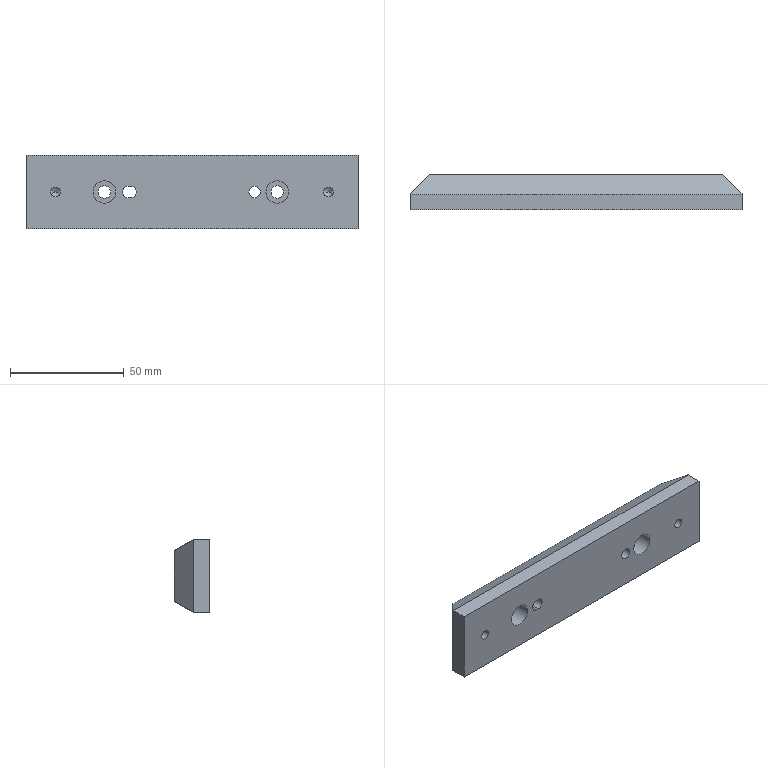NC program | NX | posted with a generic post | part box 146 x 15.5 x 32.5 mm
Whole program:
N10 G17 G21 G94 G90
(FLOOR_WALL , TOOL : D80)
N12 T19 M6
N14 G54
N16 G17 G0 G90 X-45. Y-16.25 S6500 M3
N18 G43 Z30. H19
N20 Z3.
N22 G94 G1 Z0. F1500.
N24 X-42.
N26 X188.
N28 X191.
N30 Z3.
N32 G0 Z30.
N34 M5
(ZLEVEL_PROFILE , TOOL : D10)
N36 T15 M6
N38 G54
N40 G17 G0 G90 X-1.436 Y-37.381 S9500 M3
N42 G43 Z30. H15
N44 Z1.5
N46 G94 G1 X-1.898 Y-37.266 Z1.475 F1000.
N48 X-3.104 Y-36.584 Z1.402
N50 X-4.084 Y-35.604 Z1.33
N52 X-4.766 Y-34.398 Z1.257
N54 X-5.1 Y-33.054 Z1.185
N56 Y0.554 Z-0.577
N58 X-4.766 Y1.898 Z-0.649
N60 X-4.084 Y3.104 Z-0.722
N62 X-3.104 Y4.084 Z-0.795
N64 X-1.898 Y4.766 Z-0.867
N66 X-0.554 Y5.1 Z-0.94
N68 X0. Z-0.969
N70 X146. F3000.
N72 G2 X151.1 Y0. R5.1
N74 G1 Y-32.5
N76 G2 X146. Y-37.6 R5.1
N78 G1 X0.
N80 G2 X-5.1 Y-32.5 R5.1
N82 G1 Y0.
N84 G2 X0. Y5.1 R5.1
N86 G1 X146. Z-1.332
N88 X146.5 Y5.075 Z-1.334
N90 X146.995 Y5.002 Z-1.335
N92 X147.48 Y4.88 Z-1.336
N94 X147.952 Y4.712 Z-1.337
N96 X148.404 Y4.498 Z-1.339
N98 X148.833 Y4.24 Z-1.34
N100 X149.235 Y3.942 Z-1.341
N102 X149.606 Y3.606 Z-1.342
N104 X149.942 Y3.235 Z-1.344
N106 X150.24 Y2.833 Z-1.345
N108 X150.498 Y2.404 Z-1.346
N110 X150.712 Y1.952 Z-1.347
N112 X150.88 Y1.48 Z-1.349
N114 X151.002 Y0.995 Z-1.35
N116 X151.075 Y0.5 Z-1.351
N118 X151.1 Y0. Z-1.352
N120 Y-32.5 Z-1.433
N122 X151.075 Y-33. Z-1.434
N124 X151.002 Y-33.495 Z-1.436
N126 X150.88 Y-33.98 Z-1.437
N128 X150.712 Y-34.452 Z-1.438
N130 X150.498 Y-34.904 Z-1.439
N132 X150.24 Y-35.333 Z-1.441
N134 X149.942 Y-35.735 Z-1.442
N136 X149.606 Y-36.106 Z-1.443
N138 X149.235 Y-36.442 Z-1.444
N140 X148.833 Y-36.74 Z-1.446
N142 X148.404 Y-36.998 Z-1.447
N144 X147.952 Y-37.212 Z-1.448
N146 X147.48 Y-37.38 Z-1.449
N148 X146.995 Y-37.502 Z-1.451
N150 X146.5 Y-37.575 Z-1.452
N152 X146. Y-37.6 Z-1.453
N154 X0. Z-1.817
N156 X-0.5 Y-37.575 Z-1.818
N158 X-0.995 Y-37.502 Z-1.819
N160 X-1.48 Y-37.38 Z-1.82
N162 X-1.952 Y-37.212 Z-1.822
N164 X-2.404 Y-36.998 Z-1.823
N166 X-2.833 Y-36.74 Z-1.824
N168 X-3.235 Y-36.442 Z-1.825
N170 X-3.606 Y-36.106 Z-1.827
N172 X-3.942 Y-35.735 Z-1.828
N174 X-4.24 Y-35.333 Z-1.829
N176 X-4.498 Y-34.904 Z-1.83
N178 X-4.712 Y-34.452 Z-1.832
N180 X-4.88 Y-33.98 Z-1.833
N182 X-5.002 Y-33.495 Z-1.834
N184 X-5.075 Y-33. Z-1.835
N186 X-5.1 Y-32.5 Z-1.837
N188 Y0. Z-1.918
N190 X-5.075 Y0.5 Z-1.919
N192 X-5.002 Y0.995 Z-1.92
N194 X-4.88 Y1.48 Z-1.921
N196 X-4.712 Y1.952 Z-1.923
N198 X-4.498 Y2.404 Z-1.924
N200 X-4.24 Y2.833 Z-1.925
N202 X-3.942 Y3.235 Z-1.926
N204 X-3.606 Y3.606 Z-1.928
N206 X-3.235 Y3.942 Z-1.929
N208 X-2.833 Y4.24 Z-1.93
N210 X-2.404 Y4.498 Z-1.931
N212 X-1.952 Y4.712 Z-1.933
N214 X-1.48 Y4.88 Z-1.934
N216 X-0.995 Y5.002 Z-1.935
N218 X-0.5 Y5.075 Z-1.936
N220 X0. Y5.1 Z-1.938
N222 X146. Z-2.301
N224 X146.5 Y5.075 Z-2.302
N226 X146.995 Y5.002 Z-2.304
N228 X147.48 Y4.88 Z-2.305
N230 X147.952 Y4.712 Z-2.306
N232 X148.404 Y4.498 Z-2.307
N234 X148.833 Y4.24 Z-2.309
N236 X149.235 Y3.942 Z-2.31
N238 X149.606 Y3.606 Z-2.311
N240 X149.942 Y3.235 Z-2.312
N242 X150.24 Y2.833 Z-2.314
N244 X150.498 Y2.404 Z-2.315
N246 X150.712 Y1.952 Z-2.316
N248 X150.88 Y1.48 Z-2.317
N250 X151.002 Y0.995 Z-2.319
N252 X151.075 Y0.5 Z-2.32
N254 X151.1 Y0. Z-2.321
N256 Y-32.5 Z-2.402
N258 X151.075 Y-33. Z-2.403
N260 X151.002 Y-33.495 Z-2.404
N262 X150.88 Y-33.98 Z-2.406
N264 X150.712 Y-34.452 Z-2.407
N266 X150.498 Y-34.904 Z-2.408
N268 X150.24 Y-35.333 Z-2.409
N270 X149.942 Y-35.735 Z-2.411
N272 X149.606 Y-36.106 Z-2.412
N274 X149.235 Y-36.442 Z-2.413
N276 X148.833 Y-36.74 Z-2.414
N278 X148.404 Y-36.998 Z-2.416
N280 X147.952 Y-37.212 Z-2.417
N282 X147.48 Y-37.38 Z-2.418
N284 X146.995 Y-37.502 Z-2.419
N286 X146.5 Y-37.575 Z-2.421
N288 X146. Y-37.6 Z-2.422
N290 X0. Z-2.785
N292 X-0.5 Y-37.575 Z-2.787
N294 X-0.995 Y-37.502 Z-2.788
N296 X-1.48 Y-37.38 Z-2.789
N298 X-1.952 Y-37.212 Z-2.79
N300 X-2.404 Y-36.998 Z-2.792
N302 X-2.833 Y-36.74 Z-2.793
N304 X-3.235 Y-36.442 Z-2.794
N306 X-3.606 Y-36.106 Z-2.795
N308 X-3.942 Y-35.735 Z-2.797
N310 X-4.24 Y-35.333 Z-2.798
N312 X-4.498 Y-34.904 Z-2.799
N314 X-4.712 Y-34.452 Z-2.8
N316 X-4.88 Y-33.98 Z-2.802
N318 X-5.002 Y-33.495 Z-2.803
N320 X-5.075 Y-33. Z-2.804
N322 X-5.1 Y-32.5 Z-2.805
N324 Y0. Z-2.886
N326 X-5.075 Y0.5 Z-2.888
N328 X-5.002 Y0.995 Z-2.889
N330 X-4.88 Y1.48 Z-2.89
N332 X-4.712 Y1.952 Z-2.891
N334 X-4.498 Y2.404 Z-2.893
N336 X-4.24 Y2.833 Z-2.894
N338 X-3.942 Y3.235 Z-2.895
N340 X-3.606 Y3.606 Z-2.896
N342 X-3.235 Y3.942 Z-2.898
N344 X-2.833 Y4.24 Z-2.899
N346 X-2.404 Y4.498 Z-2.9
N348 X-1.952 Y4.712 Z-2.901
N350 X-1.48 Y4.88 Z-2.903
N352 X-0.995 Y5.002 Z-2.904
N354 X-0.5 Y5.075 Z-2.905
N356 X0. Y5.1 Z-2.906
N358 X146. Z-3.27
N360 X146.5 Y5.075 Z-3.271
N362 X146.995 Y5.002 Z-3.272
N364 X147.48 Y4.88 Z-3.274
N366 X147.952 Y4.712 Z-3.275
N368 X148.404 Y4.498 Z-3.276
N370 X148.833 Y4.24 Z-3.277
N372 X149.235 Y3.942 Z-3.279
N374 X149.606 Y3.606 Z-3.28
N376 X149.942 Y3.235 Z-3.281
N378 X150.24 Y2.833 Z-3.282
N380 X150.498 Y2.404 Z-3.284
N382 X150.712 Y1.952 Z-3.285
N384 X150.88 Y1.48 Z-3.286
N386 X151.002 Y0.995 Z-3.287
N388 X151.075 Y0.5 Z-3.289
N390 X151.1 Y0. Z-3.29
N392 Y-32.5 Z-3.371
N394 X151.075 Y-33. Z-3.372
N396 X151.002 Y-33.495 Z-3.373
N398 X150.88 Y-33.98 Z-3.374
N400 X150.712 Y-34.452 Z-3.376
N402 X150.498 Y-34.904 Z-3.377
N404 X150.24 Y-35.333 Z-3.378
N406 X149.942 Y-35.735 Z-3.379
N408 X149.606 Y-36.106 Z-3.381
N410 X149.235 Y-36.442 Z-3.382
N412 X148.833 Y-36.74 Z-3.383
N414 X148.404 Y-36.998 Z-3.384
N416 X147.952 Y-37.212 Z-3.386
N418 X147.48 Y-37.38 Z-3.387
N420 X146.995 Y-37.502 Z-3.388
N422 X146.5 Y-37.575 Z-3.389
N424 X146. Y-37.6 Z-3.391
N426 X0. Z-3.754
N428 X-0.5 Y-37.575 Z-3.755
N430 X-0.995 Y-37.502 Z-3.757
N432 X-1.48 Y-37.38 Z-3.758
N434 X-1.952 Y-37.212 Z-3.759
N436 X-2.404 Y-36.998 Z-3.76
N438 X-2.833 Y-36.74 Z-3.762
N440 X-3.235 Y-36.442 Z-3.763
N442 X-3.606 Y-36.106 Z-3.764
N444 X-3.942 Y-35.735 Z-3.765
N446 X-4.24 Y-35.333 Z-3.767
N448 X-4.498 Y-34.904 Z-3.768
N450 X-4.712 Y-34.452 Z-3.769
N452 X-4.88 Y-33.98 Z-3.77
N454 X-5.002 Y-33.495 Z-3.772
N456 X-5.075 Y-33. Z-3.773
N458 X-5.1 Y-32.5 Z-3.774
N460 Y0. Z-3.855
N462 X-5.075 Y0.5 Z-3.856
N464 X-5.002 Y0.995 Z-3.858
N466 X-4.88 Y1.48 Z-3.859
N468 X-4.712 Y1.952 Z-3.86
N470 X-4.498 Y2.404 Z-3.861
N472 X-4.24 Y2.833 Z-3.863
N474 X-3.942 Y3.235 Z-3.864
N476 X-3.606 Y3.606 Z-3.865
N478 X-3.235 Y3.942 Z-3.866
N480 X-2.833 Y4.24 Z-3.868
N482 X-2.404 Y4.498 Z-3.869
N484 X-1.952 Y4.712 Z-3.87
N486 X-1.48 Y4.88 Z-3.871
N488 X-0.995 Y5.002 Z-3.873
N490 X-0.5 Y5.075 Z-3.874
N492 X0. Y5.1 Z-3.875
N494 X146. Z-4.239
N496 X146.5 Y5.075 Z-4.24
N498 X146.995 Y5.002 Z-4.241
N500 X147.48 Y4.88 Z-4.242
N502 X147.952 Y4.712 Z-4.244
N504 X148.404 Y4.498 Z-4.245
N506 X148.833 Y4.24 Z-4.246
N508 X149.235 Y3.942 Z-4.247
N510 X149.606 Y3.606 Z-4.249
N512 X149.942 Y3.235 Z-4.25
N514 X150.24 Y2.833 Z-4.251
N516 X150.498 Y2.404 Z-4.252
N518 X150.712 Y1.952 Z-4.254
N520 X150.88 Y1.48 Z-4.255
N522 X151.002 Y0.995 Z-4.256
N524 X151.075 Y0.5 Z-4.257
N526 X151.1 Y0. Z-4.259
N528 Y-32.5 Z-4.339
N530 X151.075 Y-33. Z-4.341
N532 X151.002 Y-33.495 Z-4.342
N534 X150.88 Y-33.98 Z-4.343
N536 X150.712 Y-34.452 Z-4.344
N538 X150.498 Y-34.904 Z-4.346
N540 X150.24 Y-35.333 Z-4.347
N542 X149.942 Y-35.735 Z-4.348
N544 X149.606 Y-36.106 Z-4.349
N546 X149.235 Y-36.442 Z-4.351
N548 X148.833 Y-36.74 Z-4.352
N550 X148.404 Y-36.998 Z-4.353
N552 X147.952 Y-37.212 Z-4.354
N554 X147.48 Y-37.38 Z-4.356
N556 X146.995 Y-37.502 Z-4.357
N558 X146.5 Y-37.575 Z-4.358
N560 X146. Y-37.6 Z-4.359
N562 X0. Z-4.723
N564 X-0.5 Y-37.575 Z-4.724
N566 X-0.995 Y-37.502 Z-4.725
N568 X-1.48 Y-37.38 Z-4.727
N570 X-1.952 Y-37.212 Z-4.728
N572 X-2.404 Y-36.998 Z-4.729
N574 X-2.833 Y-36.74 Z-4.73
N576 X-3.235 Y-36.442 Z-4.732
N578 X-3.606 Y-36.106 Z-4.733
N580 X-3.942 Y-35.735 Z-4.734
N582 X-4.24 Y-35.333 Z-4.735
N584 X-4.498 Y-34.904 Z-4.737
N586 X-4.712 Y-34.452 Z-4.738
N588 X-4.88 Y-33.98 Z-4.739
N590 X-5.002 Y-33.495 Z-4.74
N592 X-5.075 Y-33. Z-4.742
N594 X-5.1 Y-32.5 Z-4.743
N596 Y0. Z-4.824
N598 X-5.075 Y0.5 Z-4.825
N600 X-5.002 Y0.995 Z-4.826
N602 X-4.88 Y1.48 Z-4.828
N604 X-4.712 Y1.952 Z-4.829
N606 X-4.498 Y2.404 Z-4.83
N608 X-4.24 Y2.833 Z-4.831
N610 X-3.942 Y3.235 Z-4.833
N612 X-3.606 Y3.606 Z-4.834
N614 X-3.235 Y3.942 Z-4.835
N616 X-2.833 Y4.24 Z-4.836
N618 X-2.404 Y4.498 Z-4.838
N620 X-1.952 Y4.712 Z-4.839
N622 X-1.48 Y4.88 Z-4.84
N624 X-0.995 Y5.002 Z-4.841
N626 X-0.5 Y5.075 Z-4.843
N628 X0. Y5.1 Z-4.844
N630 X146. Z-5.207
N632 X146.5 Y5.075 Z-5.209
N634 X146.995 Y5.002 Z-5.21
N636 X147.48 Y4.88 Z-5.211
N638 X147.952 Y4.712 Z-5.212
N640 X148.404 Y4.498 Z-5.214
N642 X148.833 Y4.24 Z-5.215
N644 X149.235 Y3.942 Z-5.216
N646 X149.606 Y3.606 Z-5.217
N648 X149.942 Y3.235 Z-5.219
N650 X150.24 Y2.833 Z-5.22
N652 X150.498 Y2.404 Z-5.221
N654 X150.712 Y1.952 Z-5.222
N656 X150.88 Y1.48 Z-5.224
N658 X151.002 Y0.995 Z-5.225
N660 X151.075 Y0.5 Z-5.226
N662 X151.1 Y0. Z-5.227
N664 Y-32.5 Z-5.308
N666 X151.075 Y-33. Z-5.309
N668 X151.002 Y-33.495 Z-5.311
N670 X150.88 Y-33.98 Z-5.312
N672 X150.712 Y-34.452 Z-5.313
N674 X150.498 Y-34.904 Z-5.314
N676 X150.24 Y-35.333 Z-5.316
N678 X149.942 Y-35.735 Z-5.317
N680 X149.606 Y-36.106 Z-5.318
N682 X149.235 Y-36.442 Z-5.319
N684 X148.833 Y-36.74 Z-5.321
N686 X148.404 Y-36.998 Z-5.322
N688 X147.952 Y-37.212 Z-5.323
N690 X147.48 Y-37.38 Z-5.324
N692 X146.995 Y-37.502 Z-5.326
N694 X146.5 Y-37.575 Z-5.327
N696 X146. Y-37.6 Z-5.328
N698 X0. Z-5.692
N700 X-0.5 Y-37.575 Z-5.693
N702 X-0.995 Y-37.502 Z-5.694
N704 X-1.48 Y-37.38 Z-5.695
N706 X-1.952 Y-37.212 Z-5.697
N708 X-2.404 Y-36.998 Z-5.698
N710 X-2.833 Y-36.74 Z-5.699
N712 X-3.235 Y-36.442 Z-5.7
N714 X-3.606 Y-36.106 Z-5.702
N716 X-3.942 Y-35.735 Z-5.703
N718 X-4.24 Y-35.333 Z-5.704
N720 X-4.498 Y-34.904 Z-5.705
N722 X-4.712 Y-34.452 Z-5.707
N724 X-4.88 Y-33.98 Z-5.708
N726 X-5.002 Y-33.495 Z-5.709
N728 X-5.075 Y-33. Z-5.71
N730 X-5.1 Y-32.5 Z-5.712
N732 Y0. Z-5.793
N734 X-5.075 Y0.5 Z-5.794
N736 X-5.002 Y0.995 Z-5.795
N738 X-4.88 Y1.48 Z-5.796
N740 X-4.712 Y1.952 Z-5.798
N742 X-4.498 Y2.404 Z-5.799
N744 X-4.24 Y2.833 Z-5.8
N746 X-3.942 Y3.235 Z-5.801
N748 X-3.606 Y3.606 Z-5.803
N750 X-3.235 Y3.942 Z-5.804
N752 X-2.833 Y4.24 Z-5.805
N754 X-2.404 Y4.498 Z-5.806
N756 X-1.952 Y4.712 Z-5.808
N758 X-1.48 Y4.88 Z-5.809
N760 X-0.995 Y5.002 Z-5.81
N762 X-0.5 Y5.075 Z-5.811
N764 X0. Y5.1 Z-5.813
N766 X146. Z-6.176
N768 X146.5 Y5.075 Z-6.177
N770 X146.995 Y5.002 Z-6.179
N772 X147.48 Y4.88 Z-6.18
N774 X147.952 Y4.712 Z-6.181
N776 X148.404 Y4.498 Z-6.182
N778 X148.833 Y4.24 Z-6.184
N780 X149.235 Y3.942 Z-6.185
N782 X149.606 Y3.606 Z-6.186
N784 X149.942 Y3.235 Z-6.187
N786 X150.24 Y2.833 Z-6.189
N788 X150.498 Y2.404 Z-6.19
N790 X150.712 Y1.952 Z-6.191
N792 X150.88 Y1.48 Z-6.192
N794 X151.002 Y0.995 Z-6.194
N796 X151.075 Y0.5 Z-6.195
N798 X151.1 Y0. Z-6.196
N800 Y-32.5 Z-6.277
N802 X151.075 Y-33. Z-6.278
N804 X151.002 Y-33.495 Z-6.279
N806 X150.88 Y-33.98 Z-6.281
N808 X150.712 Y-34.452 Z-6.282
N810 X150.498 Y-34.904 Z-6.283
N812 X150.24 Y-35.333 Z-6.284
N814 X149.942 Y-35.735 Z-6.286
N816 X149.606 Y-36.106 Z-6.287
N818 X149.235 Y-36.442 Z-6.288
N820 X148.833 Y-36.74 Z-6.289
N822 X148.404 Y-36.998 Z-6.291
N824 X147.952 Y-37.212 Z-6.292
N826 X147.48 Y-37.38 Z-6.293
N828 X146.995 Y-37.502 Z-6.294
N830 X146.5 Y-37.575 Z-6.296
N832 X146. Y-37.6 Z-6.297
N834 X0. Z-6.66
N836 X-0.5 Y-37.575 Z-6.662
N838 X-0.995 Y-37.502 Z-6.663
N840 X-1.48 Y-37.38 Z-6.664
N842 X-1.952 Y-37.212 Z-6.665
N844 X-2.404 Y-36.998 Z-6.667
N846 X-2.833 Y-36.74 Z-6.668
N848 X-3.235 Y-36.442 Z-6.669
N850 X-3.606 Y-36.106 Z-6.67
N852 X-3.942 Y-35.735 Z-6.672
N854 X-4.24 Y-35.333 Z-6.673
N856 X-4.498 Y-34.904 Z-6.674
N858 X-4.712 Y-34.452 Z-6.675
N860 X-4.88 Y-33.98 Z-6.677
N862 X-5.002 Y-33.495 Z-6.678
N864 X-5.075 Y-33. Z-6.679
N866 X-5.1 Y-32.5 Z-6.68
N868 Y0. Z-6.761
N870 X-5.075 Y0.5 Z-6.763
N872 X-5.002 Y0.995 Z-6.764
N874 X-4.88 Y1.48 Z-6.765
N876 X-4.712 Y1.952 Z-6.766
N878 X-4.498 Y2.404 Z-6.768
N880 X-4.24 Y2.833 Z-6.769
N882 X-3.942 Y3.235 Z-6.77
N884 X-3.606 Y3.606 Z-6.771
N886 X-3.235 Y3.942 Z-6.773
N888 X-2.833 Y4.24 Z-6.774
N890 X-2.404 Y4.498 Z-6.775
N892 X-1.952 Y4.712 Z-6.776
N894 X-1.48 Y4.88 Z-6.778
N896 X-0.995 Y5.002 Z-6.779
N898 X-0.5 Y5.075 Z-6.78
N900 X0. Y5.1 Z-6.781
N902 X146. Z-7.145
N904 X146.5 Y5.075 Z-7.146
N906 X146.995 Y5.002 Z-7.147
N908 X147.48 Y4.88 Z-7.149
N910 X147.952 Y4.712 Z-7.15
N912 X148.404 Y4.498 Z-7.151
N914 X148.833 Y4.24 Z-7.152
N916 X149.235 Y3.942 Z-7.154
N918 X149.606 Y3.606 Z-7.155
N920 X149.942 Y3.235 Z-7.156
N922 X150.24 Y2.833 Z-7.157
N924 X150.498 Y2.404 Z-7.159
N926 X150.712 Y1.952 Z-7.16
N928 X150.88 Y1.48 Z-7.161
N930 X151.002 Y0.995 Z-7.162
N932 X151.075 Y0.5 Z-7.164
N934 X151.1 Y0. Z-7.165
N936 Y-32.5 Z-7.246
N938 X151.075 Y-33. Z-7.247
N940 X151.002 Y-33.495 Z-7.248
N942 X150.88 Y-33.98 Z-7.249
N944 X150.712 Y-34.452 Z-7.251
N946 X150.498 Y-34.904 Z-7.252
N948 X150.24 Y-35.333 Z-7.253
N950 X149.942 Y-35.735 Z-7.254
N952 X149.606 Y-36.106 Z-7.256
N954 X149.235 Y-36.442 Z-7.257
N956 X148.833 Y-36.74 Z-7.258
N958 X148.404 Y-36.998 Z-7.259
N960 X147.952 Y-37.212 Z-7.261
N962 X147.48 Y-37.38 Z-7.262
N964 X146.995 Y-37.502 Z-7.263
N966 X146.5 Y-37.575 Z-7.264
N968 X146. Y-37.6 Z-7.266
N970 X0. Z-7.629
N972 X-0.5 Y-37.575 Z-7.63
N974 X-0.995 Y-37.502 Z-7.632
N976 X-1.48 Y-37.38 Z-7.633
N978 X-1.952 Y-37.212 Z-7.634
N980 X-2.404 Y-36.998 Z-7.635
N982 X-2.833 Y-36.74 Z-7.637
N984 X-3.235 Y-36.442 Z-7.638
N986 X-3.606 Y-36.106 Z-7.639
N988 X-3.942 Y-35.735 Z-7.64
N990 X-4.24 Y-35.333 Z-7.642
N992 X-4.498 Y-34.904 Z-7.643
N994 X-4.712 Y-34.452 Z-7.644
N996 X-4.88 Y-33.98 Z-7.645
N998 X-5.002 Y-33.495 Z-7.647
N1000 X-5.075 Y-33. Z-7.648
N1002 X-5.1 Y-32.5 Z-7.649
N1004 Y0. Z-7.73
N1006 X-5.075 Y0.5 Z-7.731
N1008 X-5.002 Y0.995 Z-7.733
N1010 X-4.88 Y1.48 Z-7.734
N1012 X-4.712 Y1.952 Z-7.735
N1014 X-4.498 Y2.404 Z-7.736
N1016 X-4.24 Y2.833 Z-7.738
N1018 X-3.942 Y3.235 Z-7.739
N1020 X-3.606 Y3.606 Z-7.74
N1022 X-3.235 Y3.942 Z-7.741
N1024 X-2.833 Y4.24 Z-7.743
N1026 X-2.404 Y4.498 Z-7.744
N1028 X-1.952 Y4.712 Z-7.745
N1030 X-1.48 Y4.88 Z-7.746
N1032 X-0.995 Y5.002 Z-7.748
N1034 X-0.5 Y5.075 Z-7.749
N1036 X0. Y5.1 Z-7.75
N1038 X146. Z-8.114
N1040 X146.5 Y5.075 Z-8.115
N1042 X146.995 Y5.002 Z-8.116
N1044 X147.48 Y4.88 Z-8.117
N1046 X147.952 Y4.712 Z-8.119
N1048 X148.404 Y4.498 Z-8.12
N1050 X148.833 Y4.24 Z-8.121
N1052 X149.235 Y3.942 Z-8.122
N1054 X149.606 Y3.606 Z-8.124
N1056 X149.942 Y3.235 Z-8.125
N1058 X150.24 Y2.833 Z-8.126
N1060 X150.498 Y2.404 Z-8.127
N1062 X150.712 Y1.952 Z-8.129
N1064 X150.88 Y1.48 Z-8.13
N1066 X151.002 Y0.995 Z-8.131
N1068 X151.075 Y0.5 Z-8.132
N1070 X151.1 Y0. Z-8.134
N1072 Y-32.5 Z-8.214
N1074 X151.075 Y-33. Z-8.216
N1076 X151.002 Y-33.495 Z-8.217
N1078 X150.88 Y-33.98 Z-8.218
N1080 X150.712 Y-34.452 Z-8.219
N1082 X150.498 Y-34.904 Z-8.221
N1084 X150.24 Y-35.333 Z-8.222
N1086 X149.942 Y-35.735 Z-8.223
N1088 X149.606 Y-36.106 Z-8.224
N1090 X149.235 Y-36.442 Z-8.226
N1092 X148.833 Y-36.74 Z-8.227
N1094 X148.404 Y-36.998 Z-8.228
N1096 X147.952 Y-37.212 Z-8.229
N1098 X147.48 Y-37.38 Z-8.231
N1100 X146.995 Y-37.502 Z-8.232
N1102 X146.5 Y-37.575 Z-8.233
N1104 X146. Y-37.6 Z-8.234
N1106 X0. Z-8.598
N1108 X-0.5 Y-37.575 Z-8.599
N1110 X-0.995 Y-37.502 Z-8.6
N1112 X-1.48 Y-37.38 Z-8.602
N1114 X-1.952 Y-37.212 Z-8.603
N1116 X-2.404 Y-36.998 Z-8.604
N1118 X-2.833 Y-36.74 Z-8.605
N1120 X-3.235 Y-36.442 Z-8.607
N1122 X-3.606 Y-36.106 Z-8.608
N1124 X-3.942 Y-35.735 Z-8.609
N1126 X-4.24 Y-35.333 Z-8.61
N1128 X-4.498 Y-34.904 Z-8.612
N1130 X-4.712 Y-34.452 Z-8.613
N1132 X-4.88 Y-33.98 Z-8.614
N1134 X-5.002 Y-33.495 Z-8.615
N1136 X-5.075 Y-33. Z-8.617
N1138 X-5.1 Y-32.5 Z-8.618
N1140 Y0. Z-8.699
N1142 X-5.075 Y0.5 Z-8.7
N1144 X-5.002 Y0.995 Z-8.701
N1146 X-4.88 Y1.48 Z-8.703
N1148 X-4.712 Y1.952 Z-8.704
N1150 X-4.498 Y2.404 Z-8.705
N1152 X-4.24 Y2.833 Z-8.706
N1154 X-3.942 Y3.235 Z-8.708
N1156 X-3.606 Y3.606 Z-8.709
N1158 X-3.235 Y3.942 Z-8.71
N1160 X-2.833 Y4.24 Z-8.711
N1162 X-2.404 Y4.498 Z-8.713
N1164 X-1.952 Y4.712 Z-8.714
N1166 X-1.48 Y4.88 Z-8.715
N1168 X-0.995 Y5.002 Z-8.716
N1170 X-0.5 Y5.075 Z-8.718
N1172 X0. Y5.1 Z-8.719
N1174 X146. Z-9.082
N1176 X146.5 Y5.075 Z-9.084
N1178 X146.995 Y5.002 Z-9.085
N1180 X147.48 Y4.88 Z-9.086
N1182 X147.952 Y4.712 Z-9.087
N1184 X148.404 Y4.498 Z-9.089
N1186 X148.833 Y4.24 Z-9.09
N1188 X149.235 Y3.942 Z-9.091
N1190 X149.606 Y3.606 Z-9.092
N1192 X149.942 Y3.235 Z-9.094
N1194 X150.24 Y2.833 Z-9.095
N1196 X150.498 Y2.404 Z-9.096
N1198 X150.712 Y1.952 Z-9.097
N1200 X150.88 Y1.48 Z-9.099
N1202 X151.002 Y0.995 Z-9.1
N1204 X151.075 Y0.5 Z-9.101
N1206 X151.1 Y0. Z-9.102
N1208 Y-32.5 Z-9.183
N1210 X151.075 Y-33. Z-9.184
N1212 X151.002 Y-33.495 Z-9.186
N1214 X150.88 Y-33.98 Z-9.187
N1216 X150.712 Y-34.452 Z-9.188
N1218 X150.498 Y-34.904 Z-9.189
N1220 X150.24 Y-35.333 Z-9.191
N1222 X149.942 Y-35.735 Z-9.192
N1224 X149.606 Y-36.106 Z-9.193
N1226 X149.235 Y-36.442 Z-9.194
N1228 X148.833 Y-36.74 Z-9.196
N1230 X148.404 Y-36.998 Z-9.197
N1232 X147.952 Y-37.212 Z-9.198
N1234 X147.48 Y-37.38 Z-9.199
N1236 X146.995 Y-37.502 Z-9.201
N1238 X146.5 Y-37.575 Z-9.202
N1240 X146. Y-37.6 Z-9.203
N1242 X0. Z-9.567
N1244 X-0.5 Y-37.575 Z-9.568
N1246 X-0.995 Y-37.502 Z-9.569
N1248 X-1.48 Y-37.38 Z-9.57
N1250 X-1.952 Y-37.212 Z-9.572
N1252 X-2.404 Y-36.998 Z-9.573
N1254 X-2.833 Y-36.74 Z-9.574
N1256 X-3.235 Y-36.442 Z-9.575
N1258 X-3.606 Y-36.106 Z-9.577
N1260 X-3.942 Y-35.735 Z-9.578
N1262 X-4.24 Y-35.333 Z-9.579
N1264 X-4.498 Y-34.904 Z-9.58
N1266 X-4.712 Y-34.452 Z-9.582
N1268 X-4.88 Y-33.98 Z-9.583
N1270 X-5.002 Y-33.495 Z-9.584
N1272 X-5.075 Y-33. Z-9.585
N1274 X-5.1 Y-32.5 Z-9.587
N1276 Y0. Z-9.668
N1278 X-5.075 Y0.5 Z-9.669
N1280 X-5.002 Y0.995 Z-9.67
N1282 X-4.88 Y1.48 Z-9.671
N1284 X-4.712 Y1.952 Z-9.673
N1286 X-4.498 Y2.404 Z-9.674
N1288 X-4.24 Y2.833 Z-9.675
N1290 X-3.942 Y3.235 Z-9.676
N1292 X-3.606 Y3.606 Z-9.678
N1294 X-3.235 Y3.942 Z-9.679
N1296 X-2.833 Y4.24 Z-9.68
N1298 X-2.404 Y4.498 Z-9.681
N1300 X-1.952 Y4.712 Z-9.683
N1302 X-1.48 Y4.88 Z-9.684
N1304 X-0.995 Y5.002 Z-9.685
N1306 X-0.5 Y5.075 Z-9.686
N1308 X0. Y5.1 Z-9.688
N1310 X146. Z-10.051
N1312 X146.5 Y5.075 Z-10.052
N1314 X146.995 Y5.002 Z-10.054
N1316 X147.48 Y4.88 Z-10.055
N1318 X147.952 Y4.712 Z-10.056
N1320 X148.404 Y4.498 Z-10.057
N1322 X148.833 Y4.24 Z-10.059
N1324 X149.235 Y3.942 Z-10.06
N1326 X149.606 Y3.606 Z-10.061
N1328 X149.942 Y3.235 Z-10.062
N1330 X150.24 Y2.833 Z-10.064
N1332 X150.498 Y2.404 Z-10.065
N1334 X150.712 Y1.952 Z-10.066
N1336 X150.88 Y1.48 Z-10.067
N1338 X151.002 Y0.995 Z-10.069
N1340 X151.075 Y0.5 Z-10.07
N1342 X151.1 Y0. Z-10.071
N1344 Y-32.5 Z-10.152
N1346 X151.075 Y-33. Z-10.153
N1348 X151.002 Y-33.495 Z-10.154
N1350 X150.88 Y-33.98 Z-10.156
N1352 X150.712 Y-34.452 Z-10.157
N1354 X150.498 Y-34.904 Z-10.158
N1356 X150.24 Y-35.333 Z-10.159
N1358 X149.942 Y-35.735 Z-10.161
N1360 X149.606 Y-36.106 Z-10.162
N1362 X149.235 Y-36.442 Z-10.163
N1364 X148.833 Y-36.74 Z-10.164
N1366 X148.404 Y-36.998 Z-10.166
N1368 X147.952 Y-37.212 Z-10.167
N1370 X147.48 Y-37.38 Z-10.168
N1372 X146.995 Y-37.502 Z-10.169
N1374 X146.5 Y-37.575 Z-10.171
N1376 X146. Y-37.6 Z-10.172
N1378 X0. Z-10.535
N1380 X-0.5 Y-37.575 Z-10.537
N1382 X-0.995 Y-37.502 Z-10.538
N1384 X-1.48 Y-37.38 Z-10.539
N1386 X-1.952 Y-37.212 Z-10.54
N1388 X-2.404 Y-36.998 Z-10.542
N1390 X-2.833 Y-36.74 Z-10.543
N1392 X-3.235 Y-36.442 Z-10.544
N1394 X-3.606 Y-36.106 Z-10.545
N1396 X-3.942 Y-35.735 Z-10.547
N1398 X-4.24 Y-35.333 Z-10.548
N1400 X-4.498 Y-34.904 Z-10.549
N1402 X-4.712 Y-34.452 Z-10.55
N1404 X-4.88 Y-33.98 Z-10.552
N1406 X-5.002 Y-33.495 Z-10.553
N1408 X-5.075 Y-33. Z-10.554
N1410 X-5.1 Y-32.5 Z-10.555
N1412 Y0. Z-10.636
N1414 X-5.075 Y0.5 Z-10.638
N1416 X-5.002 Y0.995 Z-10.639
N1418 X-4.88 Y1.48 Z-10.64
N1420 X-4.712 Y1.952 Z-10.641
N1422 X-4.498 Y2.404 Z-10.643
N1424 X-4.24 Y2.833 Z-10.644
N1426 X-3.942 Y3.235 Z-10.645
N1428 X-3.606 Y3.606 Z-10.646
N1430 X-3.235 Y3.942 Z-10.648
N1432 X-2.833 Y4.24 Z-10.649
N1434 X-2.404 Y4.498 Z-10.65
N1436 X-1.952 Y4.712 Z-10.651
N1438 X-1.48 Y4.88 Z-10.653
N1440 X-0.995 Y5.002 Z-10.654
N1442 X-0.5 Y5.075 Z-10.655
N1444 X0. Y5.1 Z-10.656
N1446 X146. Z-11.02
N1448 X146.5 Y5.075 Z-11.021
N1450 X146.995 Y5.002 Z-11.022
N1452 X147.48 Y4.88 Z-11.024
N1454 X147.952 Y4.712 Z-11.025
N1456 X148.404 Y4.498 Z-11.026
N1458 X148.833 Y4.24 Z-11.027
N1460 X149.235 Y3.942 Z-11.029
N1462 X149.606 Y3.606 Z-11.03
N1464 X149.942 Y3.235 Z-11.031
N1466 X150.24 Y2.833 Z-11.032
N1468 X150.498 Y2.404 Z-11.034
N1470 X150.712 Y1.952 Z-11.035
N1472 X150.88 Y1.48 Z-11.036
N1474 X151.002 Y0.995 Z-11.037
N1476 X151.075 Y0.5 Z-11.039
N1478 X151.1 Y0. Z-11.04
N1480 Y-32.5 Z-11.121
N1482 X151.075 Y-33. Z-11.122
N1484 X151.002 Y-33.495 Z-11.123
N1486 X150.88 Y-33.98 Z-11.124
N1488 X150.712 Y-34.452 Z-11.126
N1490 X150.498 Y-34.904 Z-11.127
N1492 X150.24 Y-35.333 Z-11.128
N1494 X149.942 Y-35.735 Z-11.129
N1496 X149.606 Y-36.106 Z-11.131
N1498 X149.235 Y-36.442 Z-11.132
N1500 X148.833 Y-36.74 Z-11.133
N1502 X148.404 Y-36.998 Z-11.134
N1504 X147.952 Y-37.212 Z-11.136
N1506 X147.48 Y-37.38 Z-11.137
N1508 X146.995 Y-37.502 Z-11.138
N1510 X146.5 Y-37.575 Z-11.139
N1512 X146. Y-37.6 Z-11.141
N1514 X0. Z-11.504
N1516 X-0.5 Y-37.575 Z-11.505
N1518 X-0.995 Y-37.502 Z-11.507
N1520 X-1.48 Y-37.38 Z-11.508
N1522 X-1.952 Y-37.212 Z-11.509
N1524 X-2.404 Y-36.998 Z-11.51
N1526 X-2.833 Y-36.74 Z-11.512
N1528 X-3.235 Y-36.442 Z-11.513
N1530 X-3.606 Y-36.106 Z-11.514
N1532 X-3.942 Y-35.735 Z-11.515
N1534 X-4.24 Y-35.333 Z-11.517
N1536 X-4.498 Y-34.904 Z-11.518
N1538 X-4.712 Y-34.452 Z-11.519
N1540 X-4.88 Y-33.98 Z-11.52
N1542 X-5.002 Y-33.495 Z-11.522
N1544 X-5.075 Y-33. Z-11.523
N1546 X-5.1 Y-32.5 Z-11.524
N1548 Y0. Z-11.605
N1550 X-5.075 Y0.5 Z-11.606
N1552 X-5.002 Y0.995 Z-11.608
N1554 X-4.88 Y1.48 Z-11.609
N1556 X-4.712 Y1.952 Z-11.61
N1558 X-4.498 Y2.404 Z-11.611
N1560 X-4.24 Y2.833 Z-11.613
N1562 X-3.942 Y3.235 Z-11.614
N1564 X-3.606 Y3.606 Z-11.615
N1566 X-3.235 Y3.942 Z-11.616
N1568 X-2.833 Y4.24 Z-11.618
N1570 X-2.404 Y4.498 Z-11.619
N1572 X-1.952 Y4.712 Z-11.62
N1574 X-1.48 Y4.88 Z-11.621
N1576 X-0.995 Y5.002 Z-11.623
N1578 X-0.5 Y5.075 Z-11.624
N1580 X0. Y5.1 Z-11.625
N1582 X146. Z-11.989
N1584 X146.5 Y5.075 Z-11.99
N1586 X146.995 Y5.002 Z-11.991
N1588 X147.48 Y4.88 Z-11.992
N1590 X147.952 Y4.712 Z-11.994
N1592 X148.404 Y4.498 Z-11.995
N1594 X148.833 Y4.24 Z-11.996
N1596 X149.235 Y3.942 Z-11.997
N1598 X149.606 Y3.606 Z-11.999
N1600 X149.942 Y3.235 Z-12.
N1602 X150.24 Y2.833 Z-12.001
N1604 X150.498 Y2.404 Z-12.002
N1606 X150.712 Y1.952 Z-12.004
N1608 X150.88 Y1.48 Z-12.005
N1610 X151.002 Y0.995 Z-12.006
N1612 X151.075 Y0.5 Z-12.007
N1614 X151.1 Y0. Z-12.009
N1616 Y-32.5 Z-12.089
N1618 X151.075 Y-33. Z-12.091
N1620 X151.002 Y-33.495 Z-12.092
N1622 X150.88 Y-33.98 Z-12.093
N1624 X150.712 Y-34.452 Z-12.094
N1626 X150.498 Y-34.904 Z-12.096
N1628 X150.24 Y-35.333 Z-12.097
N1630 X149.942 Y-35.735 Z-12.098
N1632 X149.606 Y-36.106 Z-12.099
N1634 X149.235 Y-36.442 Z-12.101
N1636 X148.833 Y-36.74 Z-12.102
N1638 X148.404 Y-36.998 Z-12.103
N1640 X147.952 Y-37.212 Z-12.104
N1642 X147.48 Y-37.38 Z-12.106
N1644 X146.995 Y-37.502 Z-12.107
N1646 X146.5 Y-37.575 Z-12.108
N1648 X146. Y-37.6 Z-12.109
N1650 X0. Z-12.473
N1652 X-0.5 Y-37.575 Z-12.474
N1654 X-0.995 Y-37.502 Z-12.475
N1656 X-1.48 Y-37.38 Z-12.477
N1658 X-1.952 Y-37.212 Z-12.478
N1660 X-2.404 Y-36.998 Z-12.479
N1662 X-2.833 Y-36.74 Z-12.48
N1664 X-3.235 Y-36.442 Z-12.482
N1666 X-3.606 Y-36.106 Z-12.483
N1668 X-3.942 Y-35.735 Z-12.484
N1670 X-4.24 Y-35.333 Z-12.485
N1672 X-4.498 Y-34.904 Z-12.487
N1674 X-4.712 Y-34.452 Z-12.488
N1676 X-4.88 Y-33.98 Z-12.489
N1678 X-5.002 Y-33.495 Z-12.49
N1680 X-5.075 Y-33. Z-12.492
N1682 X-5.1 Y-32.5 Z-12.493
N1684 Y0. Z-12.574
N1686 X-5.075 Y0.5 Z-12.575
N1688 X-5.002 Y0.995 Z-12.576
N1690 X-4.88 Y1.48 Z-12.578
N1692 X-4.712 Y1.952 Z-12.579
N1694 X-4.498 Y2.404 Z-12.58
N1696 X-4.24 Y2.833 Z-12.581
N1698 X-3.942 Y3.235 Z-12.583
N1700 X-3.606 Y3.606 Z-12.584
N1702 X-3.235 Y3.942 Z-12.585
N1704 X-2.833 Y4.24 Z-12.586
N1706 X-2.404 Y4.498 Z-12.588
N1708 X-1.952 Y4.712 Z-12.589
N1710 X-1.48 Y4.88 Z-12.59
N1712 X-0.995 Y5.002 Z-12.591
N1714 X-0.5 Y5.075 Z-12.593
N1716 X0. Y5.1 Z-12.594
N1718 X146. Z-12.957
N1720 X146.5 Y5.075 Z-12.959
N1722 X146.995 Y5.002 Z-12.96
N1724 X147.48 Y4.88 Z-12.961
N1726 X147.952 Y4.712 Z-12.962
N1728 X148.404 Y4.498 Z-12.964
N1730 X148.833 Y4.24 Z-12.965
N1732 X149.235 Y3.942 Z-12.966
N1734 X149.606 Y3.606 Z-12.967
N1736 X149.942 Y3.235 Z-12.969
N1738 X150.24 Y2.833 Z-12.97
N1740 X150.498 Y2.404 Z-12.971
N1742 X150.712 Y1.952 Z-12.972
N1744 X150.88 Y1.48 Z-12.974
N1746 X151.002 Y0.995 Z-12.975
N1748 X151.075 Y0.5 Z-12.976
N1750 X151.1 Y0. Z-12.977
N1752 Y-32.5 Z-13.058
N1754 X151.075 Y-33. Z-13.059
N1756 X151.002 Y-33.495 Z-13.061
N1758 X150.88 Y-33.98 Z-13.062
N1760 X150.712 Y-34.452 Z-13.063
N1762 X150.498 Y-34.904 Z-13.064
N1764 X150.24 Y-35.333 Z-13.066
N1766 X149.942 Y-35.735 Z-13.067
N1768 X149.606 Y-36.106 Z-13.068
N1770 X149.235 Y-36.442 Z-13.069
N1772 X148.833 Y-36.74 Z-13.071
N1774 X148.404 Y-36.998 Z-13.072
N1776 X147.952 Y-37.212 Z-13.073
N1778 X147.48 Y-37.38 Z-13.074
N1780 X146.995 Y-37.502 Z-13.076
N1782 X146.5 Y-37.575 Z-13.077
N1784 X146. Y-37.6 Z-13.078
N1786 X0. Z-13.442
N1788 X-0.5 Y-37.575 Z-13.443
N1790 X-0.995 Y-37.502 Z-13.444
N1792 X-1.48 Y-37.38 Z-13.445
N1794 X-1.952 Y-37.212 Z-13.447
N1796 X-2.404 Y-36.998 Z-13.448
N1798 X-2.833 Y-36.74 Z-13.449
N1800 X-3.235 Y-36.442 Z-13.45
N1802 X-3.606 Y-36.106 Z-13.452
N1804 X-3.942 Y-35.735 Z-13.453
N1806 X-4.24 Y-35.333 Z-13.454
N1808 X-4.498 Y-34.904 Z-13.455
N1810 X-4.712 Y-34.452 Z-13.457
N1812 X-4.88 Y-33.98 Z-13.458
N1814 X-5.002 Y-33.495 Z-13.459
N1816 X-5.075 Y-33. Z-13.46
N1818 X-5.1 Y-32.5 Z-13.462
N1820 Y0. Z-13.543
N1822 X-5.075 Y0.5 Z-13.544
N1824 X-5.002 Y0.995 Z-13.545
N1826 X-4.88 Y1.48 Z-13.546
N1828 X-4.712 Y1.952 Z-13.548
N1830 X-4.498 Y2.404 Z-13.549
N1832 X-4.24 Y2.833 Z-13.55
N1834 X-3.942 Y3.235 Z-13.551
N1836 X-3.606 Y3.606 Z-13.553
N1838 X-3.235 Y3.942 Z-13.554
N1840 X-2.833 Y4.24 Z-13.555
N1842 X-2.404 Y4.498 Z-13.556
N1844 X-1.952 Y4.712 Z-13.558
N1846 X-1.48 Y4.88 Z-13.559
N1848 X-0.995 Y5.002 Z-13.56
N1850 X-0.5 Y5.075 Z-13.561
N1852 X0. Y5.1 Z-13.563
N1854 X146. Z-13.926
N1856 X146.5 Y5.075 Z-13.927
N1858 X146.995 Y5.002 Z-13.929
N1860 X147.48 Y4.88 Z-13.93
N1862 X147.952 Y4.712 Z-13.931
N1864 X148.404 Y4.498 Z-13.932
N1866 X148.833 Y4.24 Z-13.934
N1868 X149.235 Y3.942 Z-13.935
N1870 X149.606 Y3.606 Z-13.936
N1872 X149.942 Y3.235 Z-13.937
N1874 X150.24 Y2.833 Z-13.939
N1876 X150.498 Y2.404 Z-13.94
N1878 X150.712 Y1.952 Z-13.941
N1880 X150.88 Y1.48 Z-13.942
N1882 X151.002 Y0.995 Z-13.944
N1884 X151.075 Y0.5 Z-13.945
N1886 X151.1 Y0. Z-13.946
N1888 Y-32.5 Z-14.027
N1890 X151.075 Y-33. Z-14.028
N1892 X151.002 Y-33.495 Z-14.029
N1894 X150.88 Y-33.98 Z-14.031
N1896 X150.712 Y-34.452 Z-14.032
N1898 X150.498 Y-34.904 Z-14.033
N1900 X150.24 Y-35.333 Z-14.034
N1902 X149.942 Y-35.735 Z-14.036
N1904 X149.606 Y-36.106 Z-14.037
N1906 X149.235 Y-36.442 Z-14.038
N1908 X148.833 Y-36.74 Z-14.039
N1910 X148.404 Y-36.998 Z-14.041
N1912 X147.952 Y-37.212 Z-14.042
N1914 X147.48 Y-37.38 Z-14.043
N1916 X146.995 Y-37.502 Z-14.044
N1918 X146.5 Y-37.575 Z-14.046
N1920 X146. Y-37.6 Z-14.047
N1922 X0. Z-14.41
N1924 X-0.5 Y-37.575 Z-14.412
N1926 X-0.995 Y-37.502 Z-14.413
N1928 X-1.48 Y-37.38 Z-14.414
N1930 X-1.952 Y-37.212 Z-14.415
N1932 X-2.404 Y-36.998 Z-14.417
N1934 X-2.833 Y-36.74 Z-14.418
N1936 X-3.235 Y-36.442 Z-14.419
N1938 X-3.606 Y-36.106 Z-14.42
N1940 X-3.942 Y-35.735 Z-14.422
N1942 X-4.24 Y-35.333 Z-14.423
N1944 X-4.498 Y-34.904 Z-14.424
N1946 X-4.712 Y-34.452 Z-14.425
N1948 X-4.88 Y-33.98 Z-14.427
N1950 X-5.002 Y-33.495 Z-14.428
N1952 X-5.075 Y-33. Z-14.429
N1954 X-5.1 Y-32.5 Z-14.43
N1956 Y0. Z-14.511
N1958 X-5.075 Y0.5 Z-14.513
N1960 X-5.002 Y0.995 Z-14.514
N1962 X-4.88 Y1.48 Z-14.515
N1964 X-4.712 Y1.952 Z-14.516
N1966 X-4.498 Y2.404 Z-14.518
N1968 X-4.24 Y2.833 Z-14.519
N1970 X-3.942 Y3.235 Z-14.52
N1972 X-3.606 Y3.606 Z-14.521
N1974 X-3.235 Y3.942 Z-14.523
N1976 X-2.833 Y4.24 Z-14.524
N1978 X-2.404 Y4.498 Z-14.525
N1980 X-1.952 Y4.712 Z-14.526
N1982 X-1.48 Y4.88 Z-14.528
N1984 X-0.995 Y5.002 Z-14.529
N1986 X-0.5 Y5.075 Z-14.53
N1988 X0. Y5.1 Z-14.531
N1990 X146. Z-14.895
N1992 X146.5 Y5.075 Z-14.896
N1994 X146.995 Y5.002 Z-14.897
N1996 X147.48 Y4.88 Z-14.899
N1998 X147.952 Y4.712 Z-14.9
N2000 X148.404 Y4.498 Z-14.901
N2002 X148.833 Y4.24 Z-14.902
N2004 X149.235 Y3.942 Z-14.904
N2006 X149.606 Y3.606 Z-14.905
N2008 X149.942 Y3.235 Z-14.906
N2010 X150.24 Y2.833 Z-14.907
N2012 X150.498 Y2.404 Z-14.909
N2014 X150.712 Y1.952 Z-14.91
N2016 X150.88 Y1.48 Z-14.911
N2018 X151.002 Y0.995 Z-14.912
N2020 X151.075 Y0.5 Z-14.914
N2022 X151.1 Y0. Z-14.915
N2024 Y-32.5 Z-14.996
N2026 X151.075 Y-33. Z-14.997
N2028 X151.002 Y-33.495 Z-14.998
N2030 X150.88 Y-33.98 Z-14.999
N2032 X150.712 Y-34.452 Z-15.001
N2034 X150.498 Y-34.904 Z-15.002
N2036 X150.24 Y-35.333 Z-15.003
N2038 X149.942 Y-35.735 Z-15.004
N2040 X149.606 Y-36.106 Z-15.006
N2042 X149.235 Y-36.442 Z-15.007
N2044 X148.833 Y-36.74 Z-15.008
N2046 X148.404 Y-36.998 Z-15.009
N2048 X147.952 Y-37.212 Z-15.011
N2050 X147.48 Y-37.38 Z-15.012
N2052 X146.995 Y-37.502 Z-15.013
N2054 X146.5 Y-37.575 Z-15.014
N2056 X146. Y-37.6 Z-15.016
N2058 X0. Z-15.379
N2060 X-0.5 Y-37.575 Z-15.38
N2062 X-0.995 Y-37.502 Z-15.382
N2064 X-1.48 Y-37.38 Z-15.383
N2066 X-1.952 Y-37.212 Z-15.384
N2068 X-2.404 Y-36.998 Z-15.385
N2070 X-2.833 Y-36.74 Z-15.387
N2072 X-3.235 Y-36.442 Z-15.388
N2074 X-3.606 Y-36.106 Z-15.389
N2076 X-3.942 Y-35.735 Z-15.39
N2078 X-4.24 Y-35.333 Z-15.392
N2080 X-4.498 Y-34.904 Z-15.393
N2082 X-4.712 Y-34.452 Z-15.394
N2084 X-4.88 Y-33.98 Z-15.395
N2086 X-5.002 Y-33.495 Z-15.397
N2088 X-5.075 Y-33. Z-15.398
N2090 X-5.1 Y-32.5 Z-15.399
N2092 Y0. Z-15.48
N2094 X-5.075 Y0.5 Z-15.481
N2096 X-5.002 Y0.995 Z-15.483
N2098 X-4.88 Y1.48 Z-15.484
N2100 X-4.712 Y1.952 Z-15.485
N2102 X-4.498 Y2.404 Z-15.486
N2104 X-4.24 Y2.833 Z-15.488
N2106 X-3.942 Y3.235 Z-15.489
N2108 X-3.606 Y3.606 Z-15.49
N2110 X-3.235 Y3.942 Z-15.491
N2112 X-2.833 Y4.24 Z-15.493
N2114 X-2.404 Y4.498 Z-15.494
N2116 X-1.952 Y4.712 Z-15.495
N2118 X-1.48 Y4.88 Z-15.496
N2120 X-0.995 Y5.002 Z-15.498
N2122 X-0.5 Y5.075 Z-15.499
N2124 X0. Y5.1 Z-15.5
N2126 X146.
N2128 G2 X151.1 Y0. R5.1
N2130 G1 Y-32.5
N2132 G2 X146. Y-37.6 R5.1
N2134 G1 X0.
N2136 G2 X-5.1 Y-32.5 R5.1
N2138 G1 Y0.
N2140 G2 X0. Y5.1 R5.1
N2142 G1 Z-14.
N2144 G0 Z30.
N2146 M5
(ZLEVEL_PROFILE_1 , TOOL : D10JING)
N2148 T14 M6
N2150 G54
N2152 G17 G0 G90 X-1.622 Y6.809 S9500 M3
N2154 G43 Z30. H14
N2156 Z-14.
N2158 G94 G1 Z-15.5 F1000.
N2160 X-0.866 Y5.5
N2162 G3 X0. Y5. R1.
N2164 G1 X146. F1500.
N2166 G2 X151. Y0. R5.
N2168 G1 Y-32.5
N2170 G2 X146. Y-37.5 R5.
N2172 G1 X0.
N2174 G2 X-5. Y-32.5 R5.
N2176 G1 Y0.
N2178 G2 X0. Y5. R5.
N2180 G3 X0.866 Y5.5 R1.
N2182 G1 X1.732 Y7.
N2184 Z-14.
N2186 G0 Z30.
N2188 M5
(DRILLING , TOOL : D6A45)
N2190 T01 M6
N2192 G54
N2194 G17 G0 G90 X13. Y-16.25 S9500 M3
N2196 G43 Z30. H1
N2198 G94 G81 G98 Z-1. F250. R3.
N2200 X35.5
N2202 X45.5
N2204 X100.
N2206 X111.5
N2208 X133.
N2210 G80
N2212 G0 X133. Y-16.25 Z30.
N2214 M5
(DRILLING_1 , TOOL : 4.2ZT)
N2216 T04 M6
N2218 G54
N2220 G17 G0 G90 X13. Y-16.25 S2000 M3
N2222 G43 Z30. H4
N2224 G94 G83 G98 Z-13.862 F250. Q2. R3.
N2226 X45.5 Z-18.262
N2228 X100.
N2230 X133. Z-13.862
N2232 G80
N2234 G0 X133. Y-16.25 Z30.
N2236 M5
(DRILLING_1_COPY , TOOL : 5.5ZT)
N2238 T09 M6
N2240 G54
N2242 G17 G0 G90 X35.5 Y-16.25 S2000 M3
N2244 G43 Z30. H9
N2246 G94 G83 G98 Z-18.152 F250. Q2. R3.
N2248 X111.5
N2250 G80
N2252 G0 X111.5 Y-16.25 Z30.
N2254 M5
(HOLE_MILLING , TOOL : D6)
N2256 T12 M6
N2258 G54
N2260 G17 G0 G90 X35.5 Y-16.25 S9500 M3
N2262 G43 Z30. H12
N2264 Z0.5
N2266 G94 G3 X34.5 Y-15.25 R1. F1500.
N2268 X33.5 Y-16.25 R1.
N2270 X33.5 Y-16.25 Z-0.1 I2. J0.
N2272 X33.5 Y-16.25 Z-0.7 I2. J0.
N2274 X33.5 Y-16.25 Z-1.3 I2. J0.
N2276 X33.5 Y-16.25 Z-1.9 I2. J0.
N2278 X33.5 Y-16.25 Z-2.5 I2. J0.
N2280 X33.5 Y-16.25 Z-3.1 I2. J0.
N2282 X33.5 Y-16.25 Z-3.7 I2. J0.
N2284 X33.5 Y-16.25 Z-4.3 I2. J0.
N2286 X33.5 Y-16.25 Z-4.9 I2. J0.
N2288 X33.5 Y-16.25 Z-5.5 I2. J0.
N2290 X33.5 Y-16.25 Z-6.1 I2. J0.
N2292 X33.5 Y-16.25 Z-6.7 I2. J0.
N2294 X33.5 Y-16.25 Z-7.3 I2. J0.
N2296 X33.5 Y-16.25 Z-7.9 I2. J0.
N2298 X33.5 Y-16.25 Z-8.5 I2. J0.
N2300 X33.5 Y-16.25 Z-9.1 I2. J0.
N2302 X33.5 Y-16.25 Z-9.7 I2. J0.
N2304 X37.5 Y-16.25 Z-10. I2. J0.
N2306 X35.5 Y-14.25 R2.
N2308 X37.5 Y-16.25 R-2.
N2310 X36.5 Y-15.25 R1.
N2312 X35.5 Y-16.25 R1.
N2314 G0 Z30.
N2316 X111.5
N2318 Z0.5
N2320 G3 X110.5 Y-15.25 R1.
N2322 X109.5 Y-16.25 R1.
N2324 X109.5 Y-16.25 Z-0.1 I2. J0.
N2326 X109.5 Y-16.25 Z-0.7 I2. J0.
N2328 X109.5 Y-16.25 Z-1.3 I2. J0.
N2330 X109.5 Y-16.25 Z-1.9 I2. J0.
N2332 X109.5 Y-16.25 Z-2.5 I2. J0.
N2334 X109.5 Y-16.25 Z-3.1 I2. J0.
N2336 X109.5 Y-16.25 Z-3.7 I2. J0.
N2338 X109.5 Y-16.25 Z-4.3 I2. J0.
N2340 X109.5 Y-16.25 Z-4.9 I2. J0.
N2342 X109.5 Y-16.25 Z-5.5 I2. J0.
N2344 X109.5 Y-16.25 Z-6.1 I2. J0.
N2346 X109.5 Y-16.25 Z-6.7 I2. J0.
N2348 X109.5 Y-16.25 Z-7.3 I2. J0.
N2350 X109.5 Y-16.25 Z-7.9 I2. J0.
N2352 X109.5 Y-16.25 Z-8.5 I2. J0.
N2354 X109.5 Y-16.25 Z-9.1 I2. J0.
N2356 X109.5 Y-16.25 Z-9.7 I2. J0.
N2358 X113.5 Y-16.25 Z-10. I2. J0.
N2360 X111.5 Y-14.25 R2.
N2362 X113.5 Y-16.25 R-2.
N2364 X112.5 Y-15.25 R1.
N2366 X111.5 Y-16.25 R1.
N2368 G0 Z30.
N2370 M5
(PLANAR_MILL_COPY , TOOL : D6A45)
N2372 T01 M6
N2374 G54
N2376 G17 G0 G90 X133.7 Y-17.116 S9500 M3
N2378 G43 Z30. H1
N2380 Z0.5
N2382 G94 G1 Z-1. F1250.
N2384 G3 X134.2 Y-16.25 R1.
N2386 X133. Y-15.05 R1.2
N2388 X134.2 Y-16.25 R-1.2
N2390 X133.7 Y-15.384 R1.
N2392 G1 Z0.5
N2394 G0 Z30.
N2396 X112.366 Y-12.65
N2398 Z0.5
N2400 G1 Z-1.
N2402 G3 X111.5 Y-12.15 R1.
N2404 X107.4 Y-16.25 R4.1
N2406 X111.5 Y-12.15 R-4.1
N2408 X110.634 Y-12.65 R1.
N2410 G1 Z0.5
N2412 G0 Z30.
N2414 X99.634 Y-17.35
N2416 Z0.5
N2418 G1 Z-1.
N2420 G3 X100.5 Y-17.85 R1.
N2422 G1 X101.
N2424 G3 X102.6 Y-16.25 R1.6
N2426 X101. Y-14.65 R1.6
N2428 G1 X100.
N2430 G3 X98.4 Y-16.25 R1.6
N2432 X100. Y-17.85 R1.6
N2434 G1 X100.5
N2436 G3 X101.366 Y-17.35 R1.
N2438 G1 Z0.5
N2440 G0 Z30.
N2442 X73.866 Y-33.9
N2444 Z0.5
N2446 G1 Z-1.
N2448 G3 X73. Y-33.4 R1.
N2450 G1 X0.
N2452 G2 X-0.9 Y-32.5 R0.9
N2454 G1 Y0.
N2456 G2 X0. Y0.9 R0.9
N2458 G1 X146.
N2460 G2 X146.9 Y0. R0.9
N2462 G1 Y-32.5
N2464 G2 X146. Y-33.4 R0.9
N2466 G1 X73.
N2468 G3 X72.134 Y-33.9 R1.
N2470 G1 Z0.5
N2472 G0 Z30.
N2474 X44.634 Y-17.35
N2476 Z0.5
N2478 G1 Z-1.
N2480 G3 X45.5 Y-17.85 R1.
N2482 X47.1 Y-16.25 R1.6
N2484 X45.5 Y-17.85 R-1.6
N2486 X46.366 Y-17.35 R1.
N2488 G1 Z0.5
N2490 G0 Z30.
N2492 X36.366 Y-12.65
N2494 Z0.5
N2496 G1 Z-1.
N2498 G3 X35.5 Y-12.15 R1.
N2500 X31.4 Y-16.25 R4.1
N2502 X35.5 Y-12.15 R-4.1
N2504 X34.634 Y-12.65 R1.
N2506 G1 Z0.5
N2508 G0 Z30.
N2510 X12.3 Y-15.384
N2512 Z0.5
N2514 G1 Z-1.
N2516 G3 X11.8 Y-16.25 R1.
N2518 X13. Y-17.45 R1.2
N2520 X11.8 Y-16.25 R-1.2
N2522 X12.3 Y-17.116 R1.
N2524 G1 Z0.5
N2526 G0 Z30.
N2528 M5
N2530 M2